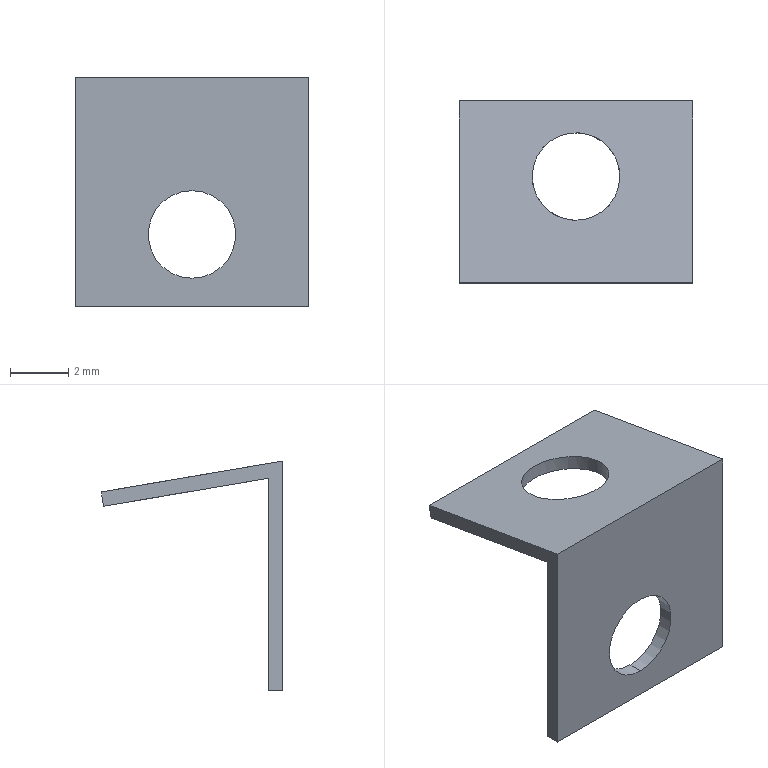Part | SolidWorks | features SplitBody 1 | 1 solid | 12 faces | box 8 x 6.232 x 7.883 mm | volume 47.269 mm3 | plane 8 | cylinder 4 | commonest cylinder face diameters 3 x4
STEP:
#1=CARTESIAN_POINT('',(43.698,45.396,-27.754));
#2=VERTEX_POINT('',#1);
#3=CARTESIAN_POINT('',(46.698,45.396,-27.754));
#4=VERTEX_POINT('',#3);
#5=CARTESIAN_POINT('',(43.698,45.396,-27.754));
#6=CARTESIAN_POINT('',(43.698,42.396,-27.243));
#7=CARTESIAN_POINT('',(46.698,42.396,-27.243));
#8=CARTESIAN_POINT('',(46.698,45.396,-27.754));
#9=(BOUNDED_CURVE()B_SPLINE_CURVE(3,(#5,#6,#7,#8),.UNSPECIFIED.,.F.,.F.)B_SPLINE_CURVE_WITH_KNOTS((4,4),(4.712,7.854),.UNSPECIFIED.)CURVE()GEOMETRIC_REPRESENTATION_ITEM()RATIONAL_B_SPLINE_CURVE((1.,0.3333,0.3333,1.))REPRESENTATION_ITEM(''));
#10=EDGE_CURVE('',#2,#4,#9,.T.);
#11=ORIENTED_EDGE('',*,*,#10,.F.);
#12=CARTESIAN_POINT('',(43.698,45.396,-27.248));
#13=VERTEX_POINT('',#12);
#14=CARTESIAN_POINT('',(43.698,45.396,-31.));
#15=DIRECTION('',(0.,0.,1.));
#16=VECTOR('',#15,1000.);
#17=LINE('',#14,#16);
#18=EDGE_CURVE('',#2,#13,#17,.T.);
#19=ORIENTED_EDGE('',*,*,#18,.T.);
#20=CARTESIAN_POINT('',(46.698,45.396,-27.248));
#21=VERTEX_POINT('',#20);
#22=CARTESIAN_POINT('',(46.698,45.396,-27.248));
#23=CARTESIAN_POINT('',(46.698,42.396,-26.738));
#24=CARTESIAN_POINT('',(43.698,42.396,-26.738));
#25=CARTESIAN_POINT('',(43.698,45.396,-27.248));
#26=(BOUNDED_CURVE()B_SPLINE_CURVE(3,(#22,#23,#24,#25),.UNSPECIFIED.,.F.,.F.)B_SPLINE_CURVE_WITH_KNOTS((4,4),(4.712,7.854),.UNSPECIFIED.)CURVE()GEOMETRIC_REPRESENTATION_ITEM()RATIONAL_B_SPLINE_CURVE((1.,0.3333,0.3333,1.))REPRESENTATION_ITEM(''));
#27=EDGE_CURVE('',#21,#13,#26,.T.);
#28=ORIENTED_EDGE('',*,*,#27,.F.);
#29=CARTESIAN_POINT('',(46.698,45.396,-31.));
#30=DIRECTION('',(0.,0.,1.));
#31=VECTOR('',#30,1000.);
#32=LINE('',#29,#31);
#33=EDGE_CURVE('',#4,#21,#32,.T.);
#34=ORIENTED_EDGE('',*,*,#33,.F.);
#35=EDGE_LOOP('',(#11,#19,#28,#34));
#36=FACE_OUTER_BOUND('',#35,.T.);
#37=CARTESIAN_POINT('',(45.198,45.396,-31.));
#38=DIRECTION('',(0.,0.,1.));
#39=DIRECTION('',(1.,0.,0.));
#40=AXIS2_PLACEMENT_3D('',#37,#38,#39);
#41=CYLINDRICAL_SURFACE('',#40,1.5);
#42=ADVANCED_FACE('',(#36),#41,.F.);
#43=CARTESIAN_POINT('',(45.198,41.756,-33.526));
#44=VERTEX_POINT('',#43);
#45=CARTESIAN_POINT('',(45.198,41.756,-30.526));
#46=VERTEX_POINT('',#45);
#47=CARTESIAN_POINT('',(45.198,41.756,-32.026));
#48=DIRECTION('',(0.,1.,0.));
#49=DIRECTION('',(0.,0.,1.));
#50=AXIS2_PLACEMENT_3D('',#47,#48,#49);
#51=CIRCLE('',#50,1.5);
#52=EDGE_CURVE('',#44,#46,#51,.T.);
#53=ORIENTED_EDGE('',*,*,#52,.F.);
#54=CARTESIAN_POINT('',(45.198,42.256,-33.526));
#55=VERTEX_POINT('',#54);
#56=CARTESIAN_POINT('',(45.198,34.256,-33.526));
#57=DIRECTION('',(0.,1.,0.));
#58=VECTOR('',#57,1000.);
#59=LINE('',#56,#58);
#60=EDGE_CURVE('',#44,#55,#59,.T.);
#61=ORIENTED_EDGE('',*,*,#60,.T.);
#62=CARTESIAN_POINT('',(45.198,42.256,-30.526));
#63=VERTEX_POINT('',#62);
#64=CARTESIAN_POINT('',(45.198,42.256,-32.026));
#65=DIRECTION('',(0.,1.,0.));
#66=DIRECTION('',(0.,0.,1.));
#67=AXIS2_PLACEMENT_3D('',#64,#65,#66);
#68=CIRCLE('',#67,1.5);
#69=EDGE_CURVE('',#55,#63,#68,.T.);
#70=ORIENTED_EDGE('',*,*,#69,.T.);
#71=CARTESIAN_POINT('',(45.198,34.256,-30.526));
#72=DIRECTION('',(0.,1.,0.));
#73=VECTOR('',#72,1000.);
#74=LINE('',#71,#73);
#75=EDGE_CURVE('',#46,#63,#74,.T.);
#76=ORIENTED_EDGE('',*,*,#75,.F.);
#77=EDGE_LOOP('',(#53,#61,#70,#76));
#78=FACE_OUTER_BOUND('',#77,.T.);
#79=CARTESIAN_POINT('',(45.198,34.256,-32.026));
#80=DIRECTION('',(0.,1.,0.));
#81=DIRECTION('',(0.,0.,1.));
#82=AXIS2_PLACEMENT_3D('',#79,#80,#81);
#83=CYLINDRICAL_SURFACE('',#82,1.5);
#84=ADVANCED_FACE('',(#78),#83,.F.);
#85=ORIENTED_EDGE('',*,*,#27,.T.);
#86=CARTESIAN_POINT('',(43.698,45.396,-27.248));
#87=CARTESIAN_POINT('',(43.698,48.396,-27.758));
#88=CARTESIAN_POINT('',(46.698,48.396,-27.758));
#89=CARTESIAN_POINT('',(46.698,45.396,-27.248));
#90=(BOUNDED_CURVE()B_SPLINE_CURVE(3,(#86,#87,#88,#89),.UNSPECIFIED.,.F.,.F.)B_SPLINE_CURVE_WITH_KNOTS((4,4),(1.571,4.712),.UNSPECIFIED.)CURVE()GEOMETRIC_REPRESENTATION_ITEM()RATIONAL_B_SPLINE_CURVE((1.,0.3333,0.3333,1.))REPRESENTATION_ITEM(''));
#91=EDGE_CURVE('',#13,#21,#90,.T.);
#92=ORIENTED_EDGE('',*,*,#91,.T.);
#93=EDGE_LOOP('',(#85,#92));
#94=FACE_BOUND('',#93,.T.);
#95=CARTESIAN_POINT('',(49.198,41.756,-26.629));
#96=VERTEX_POINT('',#95);
#97=CARTESIAN_POINT('',(49.198,47.988,-27.689));
#98=VERTEX_POINT('',#97);
#99=CARTESIAN_POINT('',(49.198,47.988,-27.689));
#100=DIRECTION('',(0.,0.9859,-0.1676));
#101=VECTOR('',#100,1000.);
#102=LINE('',#99,#101);
#103=EDGE_CURVE('',#96,#98,#102,.T.);
#104=ORIENTED_EDGE('',*,*,#103,.T.);
#105=CARTESIAN_POINT('',(41.198,47.988,-27.689));
#106=VERTEX_POINT('',#105);
#107=CARTESIAN_POINT('',(41.198,47.988,-27.689));
#108=DIRECTION('',(1.,0.,0.));
#109=VECTOR('',#108,1000.);
#110=LINE('',#107,#109);
#111=EDGE_CURVE('',#106,#98,#110,.T.);
#112=ORIENTED_EDGE('',*,*,#111,.F.);
#113=CARTESIAN_POINT('',(41.198,41.756,-26.629));
#114=VERTEX_POINT('',#113);
#115=CARTESIAN_POINT('',(41.198,47.988,-27.689));
#116=DIRECTION('',(0.,0.9859,-0.1676));
#117=VECTOR('',#116,1000.);
#118=LINE('',#115,#117);
#119=EDGE_CURVE('',#114,#106,#118,.T.);
#120=ORIENTED_EDGE('',*,*,#119,.F.);
#121=CARTESIAN_POINT('',(41.198,41.756,-26.629));
#122=DIRECTION('',(1.,0.,0.));
#123=VECTOR('',#122,1000.);
#124=LINE('',#121,#123);
#125=EDGE_CURVE('',#114,#96,#124,.T.);
#126=ORIENTED_EDGE('',*,*,#125,.T.);
#127=EDGE_LOOP('',(#104,#112,#120,#126));
#128=FACE_OUTER_BOUND('',#127,.T.);
#129=CARTESIAN_POINT('',(41.198,47.988,-27.689));
#130=DIRECTION('',(0.,-0.1676,-0.9859));
#131=DIRECTION('',(0.,0.9859,-0.1676));
#132=AXIS2_PLACEMENT_3D('',#129,#130,#131);
#133=PLANE('',#132);
#134=ADVANCED_FACE('',(#94,#128),#133,.F.);
#135=CARTESIAN_POINT('',(49.198,47.902,-28.181));
#136=VERTEX_POINT('',#135);
#137=CARTESIAN_POINT('',(49.198,47.988,-27.689));
#138=DIRECTION('',(0.,-0.1727,-0.985));
#139=VECTOR('',#138,1000.);
#140=LINE('',#137,#139);
#141=EDGE_CURVE('',#98,#136,#140,.T.);
#142=ORIENTED_EDGE('',*,*,#141,.T.);
#143=CARTESIAN_POINT('',(41.198,47.902,-28.181));
#144=VERTEX_POINT('',#143);
#145=CARTESIAN_POINT('',(41.198,47.902,-28.181));
#146=DIRECTION('',(1.,0.,0.));
#147=VECTOR('',#146,1000.);
#148=LINE('',#145,#147);
#149=EDGE_CURVE('',#144,#136,#148,.T.);
#150=ORIENTED_EDGE('',*,*,#149,.F.);
#151=CARTESIAN_POINT('',(41.198,47.988,-27.689));
#152=DIRECTION('',(0.,-0.1727,-0.985));
#153=VECTOR('',#152,1000.);
#154=LINE('',#151,#153);
#155=EDGE_CURVE('',#106,#144,#154,.T.);
#156=ORIENTED_EDGE('',*,*,#155,.F.);
#157=ORIENTED_EDGE('',*,*,#111,.T.);
#158=EDGE_LOOP('',(#142,#150,#156,#157));
#159=FACE_OUTER_BOUND('',#158,.T.);
#160=CARTESIAN_POINT('',(41.198,47.988,-27.689));
#161=DIRECTION('',(0.,-0.985,0.1727));
#162=DIRECTION('',(0.,-0.1727,-0.985));
#163=AXIS2_PLACEMENT_3D('',#160,#161,#162);
#164=PLANE('',#163);
#165=ADVANCED_FACE('',(#159),#164,.F.);
#166=CARTESIAN_POINT('',(46.698,45.396,-27.754));
#167=CARTESIAN_POINT('',(46.698,48.396,-28.265));
#168=CARTESIAN_POINT('',(43.698,48.396,-28.265));
#169=CARTESIAN_POINT('',(43.698,45.396,-27.754));
#170=(BOUNDED_CURVE()B_SPLINE_CURVE(3,(#166,#167,#168,#169),.UNSPECIFIED.,.F.,.F.)B_SPLINE_CURVE_WITH_KNOTS((4,4),(1.571,4.712),.UNSPECIFIED.)CURVE()GEOMETRIC_REPRESENTATION_ITEM()RATIONAL_B_SPLINE_CURVE((1.,0.3333,0.3333,1.))REPRESENTATION_ITEM(''));
#171=EDGE_CURVE('',#4,#2,#170,.T.);
#172=ORIENTED_EDGE('',*,*,#171,.T.);
#173=ORIENTED_EDGE('',*,*,#10,.T.);
#174=EDGE_LOOP('',(#172,#173));
#175=FACE_BOUND('',#174,.T.);
#176=CARTESIAN_POINT('',(49.198,42.256,-27.219));
#177=VERTEX_POINT('',#176);
#178=CARTESIAN_POINT('',(49.198,47.902,-28.181));
#179=DIRECTION('',(0.,-0.9858,0.1681));
#180=VECTOR('',#179,1000.);
#181=LINE('',#178,#180);
#182=EDGE_CURVE('',#136,#177,#181,.T.);
#183=ORIENTED_EDGE('',*,*,#182,.T.);
#184=CARTESIAN_POINT('',(41.198,42.256,-27.219));
#185=VERTEX_POINT('',#184);
#186=CARTESIAN_POINT('',(41.198,42.256,-27.219));
#187=DIRECTION('',(1.,0.,0.));
#188=VECTOR('',#187,1000.);
#189=LINE('',#186,#188);
#190=EDGE_CURVE('',#185,#177,#189,.T.);
#191=ORIENTED_EDGE('',*,*,#190,.F.);
#192=CARTESIAN_POINT('',(41.198,47.902,-28.181));
#193=DIRECTION('',(0.,-0.9858,0.1681));
#194=VECTOR('',#193,1000.);
#195=LINE('',#192,#194);
#196=EDGE_CURVE('',#144,#185,#195,.T.);
#197=ORIENTED_EDGE('',*,*,#196,.F.);
#198=ORIENTED_EDGE('',*,*,#149,.T.);
#199=EDGE_LOOP('',(#183,#191,#197,#198));
#200=FACE_OUTER_BOUND('',#199,.T.);
#201=CARTESIAN_POINT('',(41.198,47.902,-28.181));
#202=DIRECTION('',(0.,0.1681,0.9858));
#203=DIRECTION('',(0.,-0.9858,0.1681));
#204=AXIS2_PLACEMENT_3D('',#201,#202,#203);
#205=PLANE('',#204);
#206=ADVANCED_FACE('',(#175,#200),#205,.F.);
#207=CARTESIAN_POINT('',(45.198,42.256,-32.026));
#208=DIRECTION('',(0.,1.,0.));
#209=DIRECTION('',(0.,0.,1.));
#210=AXIS2_PLACEMENT_3D('',#207,#208,#209);
#211=CIRCLE('',#210,1.5);
#212=EDGE_CURVE('',#63,#55,#211,.T.);
#213=ORIENTED_EDGE('',*,*,#212,.F.);
#214=ORIENTED_EDGE('',*,*,#69,.F.);
#215=EDGE_LOOP('',(#213,#214));
#216=FACE_BOUND('',#215,.T.);
#217=CARTESIAN_POINT('',(49.198,42.256,-34.512));
#218=VERTEX_POINT('',#217);
#219=CARTESIAN_POINT('',(49.198,42.256,-34.512));
#220=DIRECTION('',(0.,0.,-1.));
#221=VECTOR('',#220,1000.);
#222=LINE('',#219,#221);
#223=EDGE_CURVE('',#177,#218,#222,.T.);
#224=ORIENTED_EDGE('',*,*,#223,.T.);
#225=CARTESIAN_POINT('',(41.198,42.256,-34.512));
#226=VERTEX_POINT('',#225);
#227=CARTESIAN_POINT('',(41.198,42.256,-34.512));
#228=DIRECTION('',(1.,0.,0.));
#229=VECTOR('',#228,1000.);
#230=LINE('',#227,#229);
#231=EDGE_CURVE('',#226,#218,#230,.T.);
#232=ORIENTED_EDGE('',*,*,#231,.F.);
#233=CARTESIAN_POINT('',(41.198,42.256,-34.512));
#234=DIRECTION('',(0.,0.,-1.));
#235=VECTOR('',#234,1000.);
#236=LINE('',#233,#235);
#237=EDGE_CURVE('',#185,#226,#236,.T.);
#238=ORIENTED_EDGE('',*,*,#237,.F.);
#239=ORIENTED_EDGE('',*,*,#190,.T.);
#240=EDGE_LOOP('',(#224,#232,#238,#239));
#241=FACE_OUTER_BOUND('',#240,.T.);
#242=CARTESIAN_POINT('',(41.198,42.256,-34.512));
#243=DIRECTION('',(0.,-1.,0.));
#244=DIRECTION('',(0.,0.,-1.));
#245=AXIS2_PLACEMENT_3D('',#242,#243,#244);
#246=PLANE('',#245);
#247=ADVANCED_FACE('',(#216,#241),#246,.F.);
#248=CARTESIAN_POINT('',(49.198,41.756,-34.512));
#249=VERTEX_POINT('',#248);
#250=CARTESIAN_POINT('',(49.198,42.256,-34.512));
#251=DIRECTION('',(0.,-1.,0.));
#252=VECTOR('',#251,1000.);
#253=LINE('',#250,#252);
#254=EDGE_CURVE('',#218,#249,#253,.T.);
#255=ORIENTED_EDGE('',*,*,#254,.T.);
#256=CARTESIAN_POINT('',(41.198,41.756,-34.512));
#257=VERTEX_POINT('',#256);
#258=CARTESIAN_POINT('',(41.198,41.756,-34.512));
#259=DIRECTION('',(1.,0.,0.));
#260=VECTOR('',#259,1000.);
#261=LINE('',#258,#260);
#262=EDGE_CURVE('',#257,#249,#261,.T.);
#263=ORIENTED_EDGE('',*,*,#262,.F.);
#264=CARTESIAN_POINT('',(41.198,42.256,-34.512));
#265=DIRECTION('',(0.,-1.,0.));
#266=VECTOR('',#265,1000.);
#267=LINE('',#264,#266);
#268=EDGE_CURVE('',#226,#257,#267,.T.);
#269=ORIENTED_EDGE('',*,*,#268,.F.);
#270=ORIENTED_EDGE('',*,*,#231,.T.);
#271=EDGE_LOOP('',(#255,#263,#269,#270));
#272=FACE_OUTER_BOUND('',#271,.T.);
#273=CARTESIAN_POINT('',(41.198,42.256,-34.512));
#274=DIRECTION('',(0.,0.,1.));
#275=DIRECTION('',(1.,0.,0.));
#276=AXIS2_PLACEMENT_3D('',#273,#274,#275);
#277=PLANE('',#276);
#278=ADVANCED_FACE('',(#272),#277,.F.);
#279=CARTESIAN_POINT('',(45.198,41.756,-32.026));
#280=DIRECTION('',(0.,1.,0.));
#281=DIRECTION('',(0.,0.,1.));
#282=AXIS2_PLACEMENT_3D('',#279,#280,#281);
#283=CIRCLE('',#282,1.5);
#284=EDGE_CURVE('',#46,#44,#283,.T.);
#285=ORIENTED_EDGE('',*,*,#284,.T.);
#286=ORIENTED_EDGE('',*,*,#52,.T.);
#287=EDGE_LOOP('',(#285,#286));
#288=FACE_BOUND('',#287,.T.);
#289=CARTESIAN_POINT('',(49.198,41.756,-34.512));
#290=DIRECTION('',(0.,0.,1.));
#291=VECTOR('',#290,1000.);
#292=LINE('',#289,#291);
#293=EDGE_CURVE('',#249,#96,#292,.T.);
#294=ORIENTED_EDGE('',*,*,#293,.T.);
#295=ORIENTED_EDGE('',*,*,#125,.F.);
#296=CARTESIAN_POINT('',(41.198,41.756,-34.512));
#297=DIRECTION('',(0.,0.,1.));
#298=VECTOR('',#297,1000.);
#299=LINE('',#296,#298);
#300=EDGE_CURVE('',#257,#114,#299,.T.);
#301=ORIENTED_EDGE('',*,*,#300,.F.);
#302=ORIENTED_EDGE('',*,*,#262,.T.);
#303=EDGE_LOOP('',(#294,#295,#301,#302));
#304=FACE_OUTER_BOUND('',#303,.T.);
#305=CARTESIAN_POINT('',(41.198,41.756,-34.512));
#306=DIRECTION('',(0.,1.,0.));
#307=DIRECTION('',(0.,0.,1.));
#308=AXIS2_PLACEMENT_3D('',#305,#306,#307);
#309=PLANE('',#308);
#310=ADVANCED_FACE('',(#288,#304),#309,.F.);
#311=ORIENTED_EDGE('',*,*,#119,.T.);
#312=ORIENTED_EDGE('',*,*,#155,.T.);
#313=ORIENTED_EDGE('',*,*,#196,.T.);
#314=ORIENTED_EDGE('',*,*,#237,.T.);
#315=ORIENTED_EDGE('',*,*,#268,.T.);
#316=ORIENTED_EDGE('',*,*,#300,.T.);
#317=EDGE_LOOP('',(#311,#312,#313,#314,#315,#316));
#318=FACE_OUTER_BOUND('',#317,.T.);
#319=CARTESIAN_POINT('',(41.198,0.,0.));
#320=DIRECTION('',(1.,0.,0.));
#321=DIRECTION('',(0.,0.,-1.));
#322=AXIS2_PLACEMENT_3D('',#319,#320,#321);
#323=PLANE('',#322);
#324=ADVANCED_FACE('',(#318),#323,.F.);
#325=ORIENTED_EDGE('',*,*,#103,.F.);
#326=ORIENTED_EDGE('',*,*,#293,.F.);
#327=ORIENTED_EDGE('',*,*,#254,.F.);
#328=ORIENTED_EDGE('',*,*,#223,.F.);
#329=ORIENTED_EDGE('',*,*,#182,.F.);
#330=ORIENTED_EDGE('',*,*,#141,.F.);
#331=EDGE_LOOP('',(#325,#326,#327,#328,#329,#330));
#332=FACE_OUTER_BOUND('',#331,.T.);
#333=CARTESIAN_POINT('',(49.198,0.,0.));
#334=DIRECTION('',(1.,0.,0.));
#335=DIRECTION('',(0.,0.,-1.));
#336=AXIS2_PLACEMENT_3D('',#333,#334,#335);
#337=PLANE('',#336);
#338=ADVANCED_FACE('',(#332),#337,.T.);
#339=ORIENTED_EDGE('',*,*,#60,.F.);
#340=ORIENTED_EDGE('',*,*,#284,.F.);
#341=ORIENTED_EDGE('',*,*,#75,.T.);
#342=ORIENTED_EDGE('',*,*,#212,.T.);
#343=EDGE_LOOP('',(#339,#340,#341,#342));
#344=FACE_OUTER_BOUND('',#343,.T.);
#345=CARTESIAN_POINT('',(45.198,34.256,-32.026));
#346=DIRECTION('',(0.,1.,0.));
#347=DIRECTION('',(0.,0.,1.));
#348=AXIS2_PLACEMENT_3D('',#345,#346,#347);
#349=CYLINDRICAL_SURFACE('',#348,1.5);
#350=ADVANCED_FACE('',(#344),#349,.F.);
#351=ORIENTED_EDGE('',*,*,#18,.F.);
#352=ORIENTED_EDGE('',*,*,#171,.F.);
#353=ORIENTED_EDGE('',*,*,#33,.T.);
#354=ORIENTED_EDGE('',*,*,#91,.F.);
#355=EDGE_LOOP('',(#351,#352,#353,#354));
#356=FACE_OUTER_BOUND('',#355,.T.);
#357=CARTESIAN_POINT('',(45.198,45.396,-31.));
#358=DIRECTION('',(0.,0.,1.));
#359=DIRECTION('',(1.,0.,0.));
#360=AXIS2_PLACEMENT_3D('',#357,#358,#359);
#361=CYLINDRICAL_SURFACE('',#360,1.5);
#362=ADVANCED_FACE('',(#356),#361,.F.);
#363=CLOSED_SHELL('',(#42,#84,#134,#165,#206,#247,#278,#310,#324,#338,#350,#362));
#364=MANIFOLD_SOLID_BREP('',#363);
#365=CARTESIAN_POINT('',(0.,0.,0.));
#366=DIRECTION('',(0.,0.,1.));
#367=DIRECTION('',(1.,0.,0.));
#368=AXIS2_PLACEMENT_3D('',#365,#366,#367);
#369=(LENGTH_UNIT()NAMED_UNIT(*)SI_UNIT(.MILLI.,.METRE.));
#370=UNCERTAINTY_MEASURE_WITH_UNIT(LENGTH_MEASURE(0.00001),#369,'','');
#371=(NAMED_UNIT(*)PLANE_ANGLE_UNIT()SI_UNIT($,.RADIAN.));
#372=(NAMED_UNIT(*)SI_UNIT($,.STERADIAN.)SOLID_ANGLE_UNIT());
#373=(GEOMETRIC_REPRESENTATION_CONTEXT(3)GLOBAL_UNCERTAINTY_ASSIGNED_CONTEXT((#370))GLOBAL_UNIT_ASSIGNED_CONTEXT((#369,#371,#372))REPRESENTATION_CONTEXT('',''));
#374=ADVANCED_BREP_SHAPE_REPRESENTATION('',(#364,#368),#373);